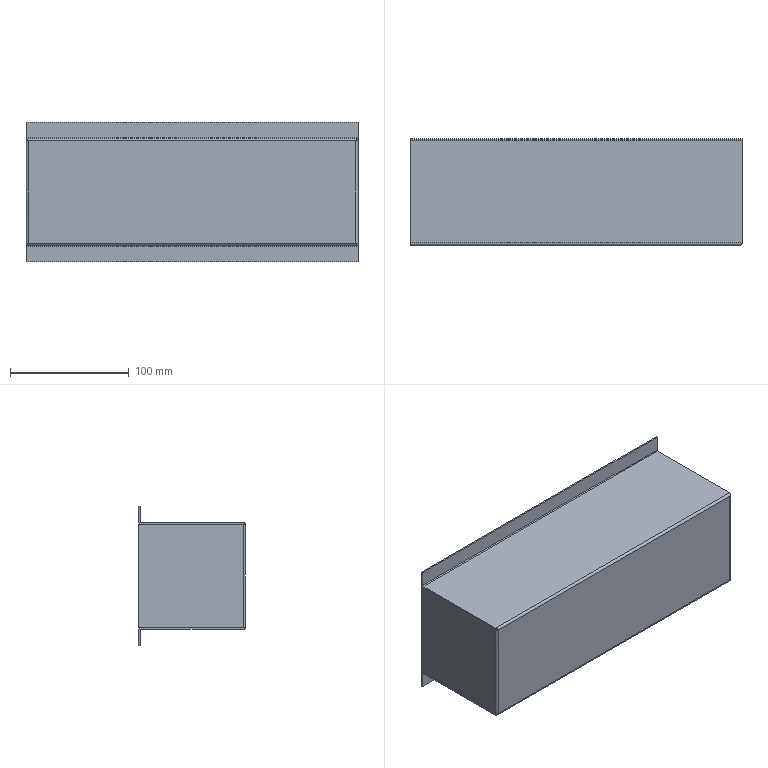Part | 1 solid | 56 faces | box 280 x 90 x 117.6 mm | volume 116674 mm3 | plane 34 | cylinder 14 | spline 8 | commonest cylinder face diameters 1.473 x6 3.873 x6 16 x2